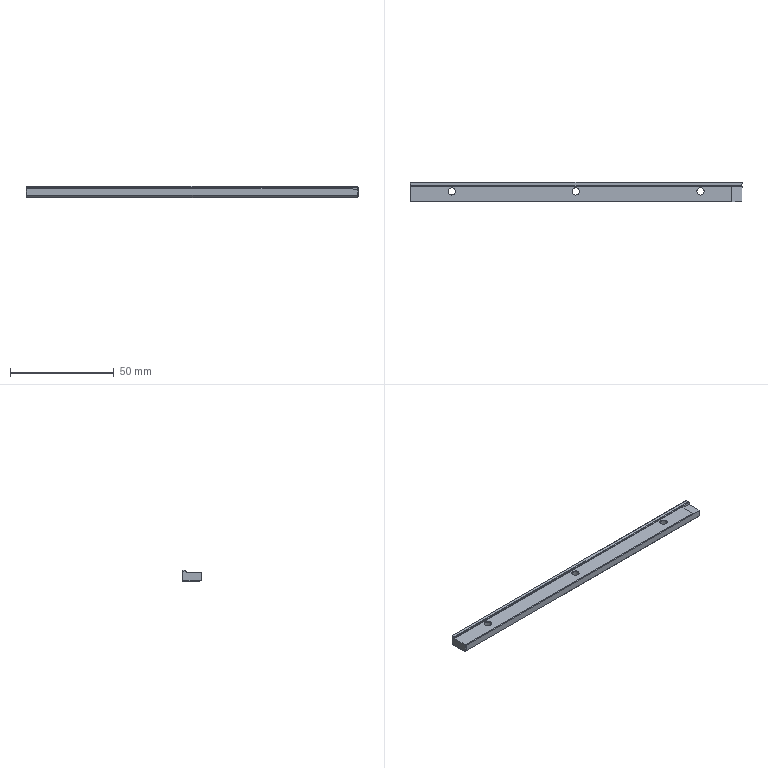Part | NX | 1 solid | 37 faces | box 159.75 x 9.6 x 5.3 mm | volume 6676 mm3 | plane 25 | cylinder 12 | commonest cylinder face diameters 3.5 x6 6 x6
STEP:
#1=CARTESIAN_POINT('',(13.59,-23.929,2.403));
#2=VERTEX_POINT('',#1);
#3=CARTESIAN_POINT('',(-145.56,-23.929,2.403));
#4=VERTEX_POINT('',#3);
#5=CARTESIAN_POINT('',(13.89,-23.929,2.403));
#6=DIRECTION('',(-1.,0.,0.));
#7=VECTOR('',#6,1000.);
#8=LINE('',#5,#7);
#9=EDGE_CURVE('',#2,#4,#8,.T.);
#10=ORIENTED_EDGE('',*,*,#9,.F.);
#11=CARTESIAN_POINT('',(13.59,-32.229,2.403));
#12=VERTEX_POINT('',#11);
#13=CARTESIAN_POINT('',(13.59,-27.929,2.403));
#14=DIRECTION('',(0.,1.,0.));
#15=VECTOR('',#14,1000.);
#16=LINE('',#13,#15);
#17=EDGE_CURVE('',#12,#2,#16,.T.);
#18=ORIENTED_EDGE('',*,*,#17,.F.);
#19=CARTESIAN_POINT('',(-145.56,-32.229,2.403));
#20=VERTEX_POINT('',#19);
#21=CARTESIAN_POINT('',(13.89,-32.229,2.403));
#22=DIRECTION('',(-1.,0.,0.));
#23=VECTOR('',#22,1000.);
#24=LINE('',#21,#23);
#25=EDGE_CURVE('',#12,#20,#24,.T.);
#26=ORIENTED_EDGE('',*,*,#25,.T.);
#27=CARTESIAN_POINT('',(-145.56,-28.079,2.403));
#28=DIRECTION('',(0.,-1.,0.));
#29=VECTOR('',#28,1000.);
#30=LINE('',#27,#29);
#31=EDGE_CURVE('',#4,#20,#30,.T.);
#32=ORIENTED_EDGE('',*,*,#31,.F.);
#33=EDGE_LOOP('',(#10,#18,#26,#32));
#34=FACE_BOUND('',#33,.T.);
#35=CARTESIAN_POINT('',(-66.11,-25.129,2.403));
#36=VERTEX_POINT('',#35);
#37=CARTESIAN_POINT('',(-66.11,-31.129,2.403));
#38=VERTEX_POINT('',#37);
#39=CARTESIAN_POINT('',(-66.11,-28.129,2.403));
#40=DIRECTION('',(0.,0.,-1.));
#41=DIRECTION('',(0.,-1.,0.));
#42=AXIS2_PLACEMENT_3D('',#39,#40,#41);
#43=CIRCLE('',#42,3.);
#44=EDGE_CURVE('',#36,#38,#43,.T.);
#45=ORIENTED_EDGE('',*,*,#44,.F.);
#46=CARTESIAN_POINT('',(-66.11,-28.129,2.403));
#47=DIRECTION('',(0.,0.,-1.));
#48=DIRECTION('',(0.,-1.,0.));
#49=AXIS2_PLACEMENT_3D('',#46,#47,#48);
#50=CIRCLE('',#49,3.);
#51=EDGE_CURVE('',#38,#36,#50,.T.);
#52=ORIENTED_EDGE('',*,*,#51,.F.);
#53=EDGE_LOOP('',(#45,#52));
#54=FACE_BOUND('',#53,.T.);
#55=CARTESIAN_POINT('',(-6.11,-25.129,2.403));
#56=VERTEX_POINT('',#55);
#57=CARTESIAN_POINT('',(-6.11,-31.129,2.403));
#58=VERTEX_POINT('',#57);
#59=CARTESIAN_POINT('',(-6.11,-28.129,2.403));
#60=DIRECTION('',(0.,0.,-1.));
#61=DIRECTION('',(0.,-1.,0.));
#62=AXIS2_PLACEMENT_3D('',#59,#60,#61);
#63=CIRCLE('',#62,3.);
#64=EDGE_CURVE('',#56,#58,#63,.T.);
#65=ORIENTED_EDGE('',*,*,#64,.F.);
#66=CARTESIAN_POINT('',(-6.11,-28.129,2.403));
#67=DIRECTION('',(0.,0.,-1.));
#68=DIRECTION('',(0.,-1.,0.));
#69=AXIS2_PLACEMENT_3D('',#66,#67,#68);
#70=CIRCLE('',#69,3.);
#71=EDGE_CURVE('',#58,#56,#70,.T.);
#72=ORIENTED_EDGE('',*,*,#71,.F.);
#73=EDGE_LOOP('',(#65,#72));
#74=FACE_BOUND('',#73,.T.);
#75=CARTESIAN_POINT('',(-125.709,-25.129,2.403));
#76=VERTEX_POINT('',#75);
#77=CARTESIAN_POINT('',(-125.709,-31.129,2.403));
#78=VERTEX_POINT('',#77);
#79=CARTESIAN_POINT('',(-125.709,-28.129,2.403));
#80=DIRECTION('',(0.,0.,-1.));
#81=DIRECTION('',(0.,-1.,0.));
#82=AXIS2_PLACEMENT_3D('',#79,#80,#81);
#83=CIRCLE('',#82,3.);
#84=EDGE_CURVE('',#76,#78,#83,.T.);
#85=ORIENTED_EDGE('',*,*,#84,.F.);
#86=CARTESIAN_POINT('',(-125.709,-28.129,2.403));
#87=DIRECTION('',(0.,0.,-1.));
#88=DIRECTION('',(0.,-1.,0.));
#89=AXIS2_PLACEMENT_3D('',#86,#87,#88);
#90=CIRCLE('',#89,3.);
#91=EDGE_CURVE('',#78,#76,#90,.T.);
#92=ORIENTED_EDGE('',*,*,#91,.F.);
#93=EDGE_LOOP('',(#85,#92));
#94=FACE_BOUND('',#93,.T.);
#95=CARTESIAN_POINT('',(13.89,-32.629,2.403));
#96=DIRECTION('',(0.,0.,-1.));
#97=DIRECTION('',(0.,-1.,0.));
#98=AXIS2_PLACEMENT_3D('',#95,#96,#97);
#99=PLANE('',#98);
#100=ADVANCED_FACE('',(#34,#54,#74,#94),#99,.T.);
#101=CARTESIAN_POINT('',(-145.56,-33.229,3.403));
#102=VERTEX_POINT('',#101);
#103=CARTESIAN_POINT('',(-145.56,-33.229,6.603));
#104=VERTEX_POINT('',#103);
#105=CARTESIAN_POINT('',(-145.56,-33.229,5.003));
#106=DIRECTION('',(0.,0.,1.));
#107=VECTOR('',#106,1000.);
#108=LINE('',#105,#107);
#109=EDGE_CURVE('',#102,#104,#108,.T.);
#110=ORIENTED_EDGE('',*,*,#109,.F.);
#111=CARTESIAN_POINT('',(13.59,-33.229,3.403));
#112=VERTEX_POINT('',#111);
#113=CARTESIAN_POINT('',(13.89,-33.229,3.403));
#114=DIRECTION('',(-1.,0.,0.));
#115=VECTOR('',#114,1000.);
#116=LINE('',#113,#115);
#117=EDGE_CURVE('',#112,#102,#116,.T.);
#118=ORIENTED_EDGE('',*,*,#117,.F.);
#119=CARTESIAN_POINT('',(13.59,-33.229,6.074));
#120=VERTEX_POINT('',#119);
#121=CARTESIAN_POINT('',(13.59,-33.229,4.712));
#122=DIRECTION('',(0.,0.,-1.));
#123=VECTOR('',#122,1000.);
#124=LINE('',#121,#123);
#125=EDGE_CURVE('',#120,#112,#124,.T.);
#126=ORIENTED_EDGE('',*,*,#125,.F.);
#127=CARTESIAN_POINT('',(10.591,-33.229,6.603));
#128=VERTEX_POINT('',#127);
#129=CARTESIAN_POINT('',(13.89,-33.229,6.021));
#130=DIRECTION('',(0.9848,0.,-0.1736));
#131=VECTOR('',#130,1000.);
#132=LINE('',#129,#131);
#133=EDGE_CURVE('',#128,#120,#132,.T.);
#134=ORIENTED_EDGE('',*,*,#133,.F.);
#135=CARTESIAN_POINT('',(13.89,-33.229,6.603));
#136=DIRECTION('',(1.,0.,0.));
#137=VECTOR('',#136,1000.);
#138=LINE('',#135,#137);
#139=EDGE_CURVE('',#104,#128,#138,.T.);
#140=ORIENTED_EDGE('',*,*,#139,.F.);
#141=EDGE_LOOP('',(#110,#118,#126,#134,#140));
#142=FACE_BOUND('',#141,.T.);
#143=CARTESIAN_POINT('',(13.89,-33.229,6.903));
#144=DIRECTION('',(0.,-1.,0.));
#145=DIRECTION('',(-1.,0.,0.));
#146=AXIS2_PLACEMENT_3D('',#143,#144,#145);
#147=PLANE('',#146);
#148=ADVANCED_FACE('',(#142),#147,.T.);
#149=CARTESIAN_POINT('',(8.89,-25.629,6.903));
#150=VERTEX_POINT('',#149);
#151=CARTESIAN_POINT('',(8.89,-32.929,6.903));
#152=VERTEX_POINT('',#151);
#153=CARTESIAN_POINT('',(8.89,-28.565,6.903));
#154=DIRECTION('',(0.,-1.,0.));
#155=VECTOR('',#154,1000.);
#156=LINE('',#153,#155);
#157=EDGE_CURVE('',#150,#152,#156,.T.);
#158=ORIENTED_EDGE('',*,*,#157,.F.);
#159=CARTESIAN_POINT('',(-145.86,-25.629,6.903));
#160=VERTEX_POINT('',#159);
#161=CARTESIAN_POINT('',(13.89,-25.629,6.903));
#162=DIRECTION('',(1.,0.,0.));
#163=VECTOR('',#162,1000.);
#164=LINE('',#161,#163);
#165=EDGE_CURVE('',#160,#150,#164,.T.);
#166=ORIENTED_EDGE('',*,*,#165,.F.);
#167=CARTESIAN_POINT('',(-145.86,-32.929,6.903));
#168=VERTEX_POINT('',#167);
#169=CARTESIAN_POINT('',(-145.86,-28.565,6.903));
#170=DIRECTION('',(0.,1.,0.));
#171=VECTOR('',#170,1000.);
#172=LINE('',#169,#171);
#173=EDGE_CURVE('',#168,#160,#172,.T.);
#174=ORIENTED_EDGE('',*,*,#173,.F.);
#175=CARTESIAN_POINT('',(13.89,-32.929,6.903));
#176=DIRECTION('',(1.,0.,0.));
#177=VECTOR('',#176,1000.);
#178=LINE('',#175,#177);
#179=EDGE_CURVE('',#168,#152,#178,.T.);
#180=ORIENTED_EDGE('',*,*,#179,.T.);
#181=EDGE_LOOP('',(#158,#166,#174,#180));
#182=FACE_BOUND('',#181,.T.);
#183=CARTESIAN_POINT('',(-125.709,-26.379,6.903));
#184=VERTEX_POINT('',#183);
#185=CARTESIAN_POINT('',(-125.709,-29.879,6.903));
#186=VERTEX_POINT('',#185);
#187=CARTESIAN_POINT('',(-125.709,-28.129,6.903));
#188=DIRECTION('',(0.,0.,-1.));
#189=DIRECTION('',(0.,-1.,0.));
#190=AXIS2_PLACEMENT_3D('',#187,#188,#189);
#191=CIRCLE('',#190,1.75);
#192=EDGE_CURVE('',#184,#186,#191,.T.);
#193=ORIENTED_EDGE('',*,*,#192,.T.);
#194=CARTESIAN_POINT('',(-125.709,-28.129,6.903));
#195=DIRECTION('',(0.,0.,-1.));
#196=DIRECTION('',(0.,-1.,0.));
#197=AXIS2_PLACEMENT_3D('',#194,#195,#196);
#198=CIRCLE('',#197,1.75);
#199=EDGE_CURVE('',#186,#184,#198,.T.);
#200=ORIENTED_EDGE('',*,*,#199,.T.);
#201=EDGE_LOOP('',(#193,#200));
#202=FACE_BOUND('',#201,.T.);
#203=CARTESIAN_POINT('',(-6.11,-26.379,6.903));
#204=VERTEX_POINT('',#203);
#205=CARTESIAN_POINT('',(-6.11,-29.879,6.903));
#206=VERTEX_POINT('',#205);
#207=CARTESIAN_POINT('',(-6.11,-28.129,6.903));
#208=DIRECTION('',(0.,0.,-1.));
#209=DIRECTION('',(0.,-1.,0.));
#210=AXIS2_PLACEMENT_3D('',#207,#208,#209);
#211=CIRCLE('',#210,1.75);
#212=EDGE_CURVE('',#204,#206,#211,.T.);
#213=ORIENTED_EDGE('',*,*,#212,.T.);
#214=CARTESIAN_POINT('',(-6.11,-28.129,6.903));
#215=DIRECTION('',(0.,0.,-1.));
#216=DIRECTION('',(0.,-1.,0.));
#217=AXIS2_PLACEMENT_3D('',#214,#215,#216);
#218=CIRCLE('',#217,1.75);
#219=EDGE_CURVE('',#206,#204,#218,.T.);
#220=ORIENTED_EDGE('',*,*,#219,.T.);
#221=EDGE_LOOP('',(#213,#220));
#222=FACE_BOUND('',#221,.T.);
#223=CARTESIAN_POINT('',(-66.11,-26.379,6.903));
#224=VERTEX_POINT('',#223);
#225=CARTESIAN_POINT('',(-66.11,-29.879,6.903));
#226=VERTEX_POINT('',#225);
#227=CARTESIAN_POINT('',(-66.11,-28.129,6.903));
#228=DIRECTION('',(0.,0.,-1.));
#229=DIRECTION('',(0.,-1.,0.));
#230=AXIS2_PLACEMENT_3D('',#227,#228,#229);
#231=CIRCLE('',#230,1.75);
#232=EDGE_CURVE('',#224,#226,#231,.T.);
#233=ORIENTED_EDGE('',*,*,#232,.T.);
#234=CARTESIAN_POINT('',(-66.11,-28.129,6.903));
#235=DIRECTION('',(0.,0.,-1.));
#236=DIRECTION('',(0.,-1.,0.));
#237=AXIS2_PLACEMENT_3D('',#234,#235,#236);
#238=CIRCLE('',#237,1.75);
#239=EDGE_CURVE('',#226,#224,#238,.T.);
#240=ORIENTED_EDGE('',*,*,#239,.T.);
#241=EDGE_LOOP('',(#233,#240));
#242=FACE_BOUND('',#241,.T.);
#243=CARTESIAN_POINT('',(13.89,-25.629,6.903));
#244=DIRECTION('',(0.,0.,1.));
#245=DIRECTION('',(1.,0.,0.));
#246=AXIS2_PLACEMENT_3D('',#243,#244,#245);
#247=PLANE('',#246);
#248=ADVANCED_FACE('',(#182,#202,#222,#242),#247,.T.);
#249=CARTESIAN_POINT('',(-145.56,-23.629,7.403));
#250=VERTEX_POINT('',#249);
#251=CARTESIAN_POINT('',(-145.56,-23.629,2.703));
#252=VERTEX_POINT('',#251);
#253=CARTESIAN_POINT('',(-145.56,-23.629,5.053));
#254=DIRECTION('',(0.,0.,-1.));
#255=VECTOR('',#254,1000.);
#256=LINE('',#253,#255);
#257=EDGE_CURVE('',#250,#252,#256,.T.);
#258=ORIENTED_EDGE('',*,*,#257,.F.);
#259=CARTESIAN_POINT('',(13.59,-23.629,7.403));
#260=VERTEX_POINT('',#259);
#261=CARTESIAN_POINT('',(13.89,-23.629,7.403));
#262=DIRECTION('',(-1.,0.,0.));
#263=VECTOR('',#262,1000.);
#264=LINE('',#261,#263);
#265=EDGE_CURVE('',#260,#250,#264,.T.);
#266=ORIENTED_EDGE('',*,*,#265,.F.);
#267=CARTESIAN_POINT('',(13.59,-23.629,2.703));
#268=VERTEX_POINT('',#267);
#269=CARTESIAN_POINT('',(13.59,-23.629,5.053));
#270=DIRECTION('',(0.,0.,1.));
#271=VECTOR('',#270,1000.);
#272=LINE('',#269,#271);
#273=EDGE_CURVE('',#268,#260,#272,.T.);
#274=ORIENTED_EDGE('',*,*,#273,.F.);
#275=CARTESIAN_POINT('',(13.89,-23.629,2.703));
#276=DIRECTION('',(-1.,0.,0.));
#277=VECTOR('',#276,1000.);
#278=LINE('',#275,#277);
#279=EDGE_CURVE('',#268,#252,#278,.T.);
#280=ORIENTED_EDGE('',*,*,#279,.T.);
#281=EDGE_LOOP('',(#258,#266,#274,#280));
#282=FACE_BOUND('',#281,.T.);
#283=CARTESIAN_POINT('',(13.89,-23.629,4.403));
#284=DIRECTION('',(0.,1.,0.));
#285=DIRECTION('',(1.,0.,0.));
#286=AXIS2_PLACEMENT_3D('',#283,#284,#285);
#287=PLANE('',#286);
#288=ADVANCED_FACE('',(#282),#287,.T.);
#289=ORIENTED_EDGE('',*,*,#64,.T.);
#290=CARTESIAN_POINT('',(-6.11,-31.129,6.403));
#291=VERTEX_POINT('',#290);
#292=CARTESIAN_POINT('',(-6.11,-31.129,3.403));
#293=DIRECTION('',(0.,0.,-1.));
#294=VECTOR('',#293,1000.);
#295=LINE('',#292,#294);
#296=EDGE_CURVE('',#58,#291,#295,.F.);
#297=ORIENTED_EDGE('',*,*,#296,.T.);
#298=CARTESIAN_POINT('',(-6.11,-25.129,6.403));
#299=VERTEX_POINT('',#298);
#300=CARTESIAN_POINT('',(-6.11,-28.129,6.403));
#301=DIRECTION('',(0.,0.,-1.));
#302=DIRECTION('',(0.,-1.,0.));
#303=AXIS2_PLACEMENT_3D('',#300,#301,#302);
#304=CIRCLE('',#303,3.);
#305=EDGE_CURVE('',#299,#291,#304,.T.);
#306=ORIENTED_EDGE('',*,*,#305,.F.);
#307=CARTESIAN_POINT('',(-6.11,-25.129,3.403));
#308=DIRECTION('',(0.,0.,-1.));
#309=VECTOR('',#308,1000.);
#310=LINE('',#307,#309);
#311=EDGE_CURVE('',#56,#299,#310,.F.);
#312=ORIENTED_EDGE('',*,*,#311,.F.);
#313=EDGE_LOOP('',(#289,#297,#306,#312));
#314=FACE_BOUND('',#313,.T.);
#315=CARTESIAN_POINT('',(-6.11,-28.129,3.403));
#316=DIRECTION('',(0.,0.,-1.));
#317=DIRECTION('',(0.,-1.,0.));
#318=AXIS2_PLACEMENT_3D('',#315,#316,#317);
#319=CYLINDRICAL_SURFACE('',#318,3.);
#320=ADVANCED_FACE('',(#314),#319,.F.);
#321=ORIENTED_EDGE('',*,*,#305,.T.);
#322=CARTESIAN_POINT('',(-6.11,-28.129,6.403));
#323=DIRECTION('',(0.,0.,-1.));
#324=DIRECTION('',(0.,-1.,0.));
#325=AXIS2_PLACEMENT_3D('',#322,#323,#324);
#326=CIRCLE('',#325,3.);
#327=EDGE_CURVE('',#291,#299,#326,.T.);
#328=ORIENTED_EDGE('',*,*,#327,.T.);
#329=EDGE_LOOP('',(#321,#328));
#330=FACE_BOUND('',#329,.T.);
#331=CARTESIAN_POINT('',(-6.11,-26.379,6.403));
#332=VERTEX_POINT('',#331);
#333=CARTESIAN_POINT('',(-6.11,-29.879,6.403));
#334=VERTEX_POINT('',#333);
#335=CARTESIAN_POINT('',(-6.11,-28.129,6.403));
#336=DIRECTION('',(0.,0.,-1.));
#337=DIRECTION('',(0.,-1.,0.));
#338=AXIS2_PLACEMENT_3D('',#335,#336,#337);
#339=CIRCLE('',#338,1.75);
#340=EDGE_CURVE('',#332,#334,#339,.T.);
#341=ORIENTED_EDGE('',*,*,#340,.F.);
#342=CARTESIAN_POINT('',(-6.11,-28.129,6.403));
#343=DIRECTION('',(0.,0.,-1.));
#344=DIRECTION('',(0.,-1.,0.));
#345=AXIS2_PLACEMENT_3D('',#342,#343,#344);
#346=CIRCLE('',#345,1.75);
#347=EDGE_CURVE('',#334,#332,#346,.T.);
#348=ORIENTED_EDGE('',*,*,#347,.F.);
#349=EDGE_LOOP('',(#341,#348));
#350=FACE_BOUND('',#349,.T.);
#351=CARTESIAN_POINT('',(-6.11,-28.129,6.403));
#352=DIRECTION('',(0.,0.,-1.));
#353=DIRECTION('',(0.,-1.,0.));
#354=AXIS2_PLACEMENT_3D('',#351,#352,#353);
#355=PLANE('',#354);
#356=ADVANCED_FACE('',(#330,#350),#355,.T.);
#357=ORIENTED_EDGE('',*,*,#340,.T.);
#358=CARTESIAN_POINT('',(-6.11,-29.879,3.403));
#359=DIRECTION('',(0.,0.,-1.));
#360=VECTOR('',#359,1000.);
#361=LINE('',#358,#360);
#362=EDGE_CURVE('',#334,#206,#361,.F.);
#363=ORIENTED_EDGE('',*,*,#362,.T.);
#364=ORIENTED_EDGE('',*,*,#212,.F.);
#365=CARTESIAN_POINT('',(-6.11,-26.379,3.403));
#366=DIRECTION('',(0.,0.,-1.));
#367=VECTOR('',#366,1000.);
#368=LINE('',#365,#367);
#369=EDGE_CURVE('',#332,#204,#368,.F.);
#370=ORIENTED_EDGE('',*,*,#369,.F.);
#371=EDGE_LOOP('',(#357,#363,#364,#370));
#372=FACE_BOUND('',#371,.T.);
#373=CARTESIAN_POINT('',(-6.11,-28.129,3.403));
#374=DIRECTION('',(0.,0.,-1.));
#375=DIRECTION('',(0.,-1.,0.));
#376=AXIS2_PLACEMENT_3D('',#373,#374,#375);
#377=CYLINDRICAL_SURFACE('',#376,1.75);
#378=ADVANCED_FACE('',(#372),#377,.F.);
#379=CARTESIAN_POINT('',(-66.11,-26.379,6.403));
#380=VERTEX_POINT('',#379);
#381=CARTESIAN_POINT('',(-66.11,-29.879,6.403));
#382=VERTEX_POINT('',#381);
#383=CARTESIAN_POINT('',(-66.11,-28.129,6.403));
#384=DIRECTION('',(0.,0.,-1.));
#385=DIRECTION('',(0.,-1.,0.));
#386=AXIS2_PLACEMENT_3D('',#383,#384,#385);
#387=CIRCLE('',#386,1.75);
#388=EDGE_CURVE('',#380,#382,#387,.T.);
#389=ORIENTED_EDGE('',*,*,#388,.T.);
#390=CARTESIAN_POINT('',(-66.11,-29.879,3.403));
#391=DIRECTION('',(0.,0.,-1.));
#392=VECTOR('',#391,1000.);
#393=LINE('',#390,#392);
#394=EDGE_CURVE('',#382,#226,#393,.F.);
#395=ORIENTED_EDGE('',*,*,#394,.T.);
#396=ORIENTED_EDGE('',*,*,#232,.F.);
#397=CARTESIAN_POINT('',(-66.11,-26.379,3.403));
#398=DIRECTION('',(0.,0.,-1.));
#399=VECTOR('',#398,1000.);
#400=LINE('',#397,#399);
#401=EDGE_CURVE('',#380,#224,#400,.F.);
#402=ORIENTED_EDGE('',*,*,#401,.F.);
#403=EDGE_LOOP('',(#389,#395,#396,#402));
#404=FACE_BOUND('',#403,.T.);
#405=CARTESIAN_POINT('',(-66.11,-28.129,3.403));
#406=DIRECTION('',(0.,0.,-1.));
#407=DIRECTION('',(0.,-1.,0.));
#408=AXIS2_PLACEMENT_3D('',#405,#406,#407);
#409=CYLINDRICAL_SURFACE('',#408,1.75);
#410=ADVANCED_FACE('',(#404),#409,.F.);
#411=CARTESIAN_POINT('',(-66.11,-25.129,6.403));
#412=VERTEX_POINT('',#411);
#413=CARTESIAN_POINT('',(-66.11,-31.129,6.403));
#414=VERTEX_POINT('',#413);
#415=CARTESIAN_POINT('',(-66.11,-28.129,6.403));
#416=DIRECTION('',(0.,0.,-1.));
#417=DIRECTION('',(0.,-1.,0.));
#418=AXIS2_PLACEMENT_3D('',#415,#416,#417);
#419=CIRCLE('',#418,3.);
#420=EDGE_CURVE('',#412,#414,#419,.T.);
#421=ORIENTED_EDGE('',*,*,#420,.T.);
#422=CARTESIAN_POINT('',(-66.11,-28.129,6.403));
#423=DIRECTION('',(0.,0.,-1.));
#424=DIRECTION('',(0.,-1.,0.));
#425=AXIS2_PLACEMENT_3D('',#422,#423,#424);
#426=CIRCLE('',#425,3.);
#427=EDGE_CURVE('',#414,#412,#426,.T.);
#428=ORIENTED_EDGE('',*,*,#427,.T.);
#429=EDGE_LOOP('',(#421,#428));
#430=FACE_BOUND('',#429,.T.);
#431=ORIENTED_EDGE('',*,*,#388,.F.);
#432=CARTESIAN_POINT('',(-66.11,-28.129,6.403));
#433=DIRECTION('',(0.,0.,-1.));
#434=DIRECTION('',(0.,-1.,0.));
#435=AXIS2_PLACEMENT_3D('',#432,#433,#434);
#436=CIRCLE('',#435,1.75);
#437=EDGE_CURVE('',#382,#380,#436,.T.);
#438=ORIENTED_EDGE('',*,*,#437,.F.);
#439=EDGE_LOOP('',(#431,#438));
#440=FACE_BOUND('',#439,.T.);
#441=CARTESIAN_POINT('',(-66.11,-28.129,6.403));
#442=DIRECTION('',(0.,0.,-1.));
#443=DIRECTION('',(0.,-1.,0.));
#444=AXIS2_PLACEMENT_3D('',#441,#442,#443);
#445=PLANE('',#444);
#446=ADVANCED_FACE('',(#430,#440),#445,.T.);
#447=ORIENTED_EDGE('',*,*,#44,.T.);
#448=CARTESIAN_POINT('',(-66.11,-31.129,3.403));
#449=DIRECTION('',(0.,0.,-1.));
#450=VECTOR('',#449,1000.);
#451=LINE('',#448,#450);
#452=EDGE_CURVE('',#38,#414,#451,.F.);
#453=ORIENTED_EDGE('',*,*,#452,.T.);
#454=ORIENTED_EDGE('',*,*,#420,.F.);
#455=CARTESIAN_POINT('',(-66.11,-25.129,3.403));
#456=DIRECTION('',(0.,0.,-1.));
#457=VECTOR('',#456,1000.);
#458=LINE('',#455,#457);
#459=EDGE_CURVE('',#36,#412,#458,.F.);
#460=ORIENTED_EDGE('',*,*,#459,.F.);
#461=EDGE_LOOP('',(#447,#453,#454,#460));
#462=FACE_BOUND('',#461,.T.);
#463=CARTESIAN_POINT('',(-66.11,-28.129,3.403));
#464=DIRECTION('',(0.,0.,-1.));
#465=DIRECTION('',(0.,-1.,0.));
#466=AXIS2_PLACEMENT_3D('',#463,#464,#465);
#467=CYLINDRICAL_SURFACE('',#466,3.);
#468=ADVANCED_FACE('',(#462),#467,.F.);
#469=CARTESIAN_POINT('',(-125.709,-26.379,6.403));
#470=VERTEX_POINT('',#469);
#471=CARTESIAN_POINT('',(-125.709,-29.879,6.403));
#472=VERTEX_POINT('',#471);
#473=CARTESIAN_POINT('',(-125.709,-28.129,6.403));
#474=DIRECTION('',(0.,0.,-1.));
#475=DIRECTION('',(0.,-1.,0.));
#476=AXIS2_PLACEMENT_3D('',#473,#474,#475);
#477=CIRCLE('',#476,1.75);
#478=EDGE_CURVE('',#470,#472,#477,.T.);
#479=ORIENTED_EDGE('',*,*,#478,.T.);
#480=CARTESIAN_POINT('',(-125.709,-29.879,3.403));
#481=DIRECTION('',(0.,0.,-1.));
#482=VECTOR('',#481,1000.);
#483=LINE('',#480,#482);
#484=EDGE_CURVE('',#472,#186,#483,.F.);
#485=ORIENTED_EDGE('',*,*,#484,.T.);
#486=ORIENTED_EDGE('',*,*,#192,.F.);
#487=CARTESIAN_POINT('',(-125.709,-26.379,3.403));
#488=DIRECTION('',(0.,0.,-1.));
#489=VECTOR('',#488,1000.);
#490=LINE('',#487,#489);
#491=EDGE_CURVE('',#470,#184,#490,.F.);
#492=ORIENTED_EDGE('',*,*,#491,.F.);
#493=EDGE_LOOP('',(#479,#485,#486,#492));
#494=FACE_BOUND('',#493,.T.);
#495=CARTESIAN_POINT('',(-125.709,-28.129,3.403));
#496=DIRECTION('',(0.,0.,-1.));
#497=DIRECTION('',(0.,-1.,0.));
#498=AXIS2_PLACEMENT_3D('',#495,#496,#497);
#499=CYLINDRICAL_SURFACE('',#498,1.75);
#500=ADVANCED_FACE('',(#494),#499,.F.);
#501=CARTESIAN_POINT('',(-125.709,-25.129,6.403));
#502=VERTEX_POINT('',#501);
#503=CARTESIAN_POINT('',(-125.709,-31.129,6.403));
#504=VERTEX_POINT('',#503);
#505=CARTESIAN_POINT('',(-125.709,-28.129,6.403));
#506=DIRECTION('',(0.,0.,-1.));
#507=DIRECTION('',(0.,-1.,0.));
#508=AXIS2_PLACEMENT_3D('',#505,#506,#507);
#509=CIRCLE('',#508,3.);
#510=EDGE_CURVE('',#502,#504,#509,.T.);
#511=ORIENTED_EDGE('',*,*,#510,.T.);
#512=CARTESIAN_POINT('',(-125.709,-28.129,6.403));
#513=DIRECTION('',(0.,0.,-1.));
#514=DIRECTION('',(0.,-1.,0.));
#515=AXIS2_PLACEMENT_3D('',#512,#513,#514);
#516=CIRCLE('',#515,3.);
#517=EDGE_CURVE('',#504,#502,#516,.T.);
#518=ORIENTED_EDGE('',*,*,#517,.T.);
#519=EDGE_LOOP('',(#511,#518));
#520=FACE_BOUND('',#519,.T.);
#521=ORIENTED_EDGE('',*,*,#478,.F.);
#522=CARTESIAN_POINT('',(-125.709,-28.129,6.403));
#523=DIRECTION('',(0.,0.,-1.));
#524=DIRECTION('',(0.,-1.,0.));
#525=AXIS2_PLACEMENT_3D('',#522,#523,#524);
#526=CIRCLE('',#525,1.75);
#527=EDGE_CURVE('',#472,#470,#526,.T.);
#528=ORIENTED_EDGE('',*,*,#527,.F.);
#529=EDGE_LOOP('',(#521,#528));
#530=FACE_BOUND('',#529,.T.);
#531=CARTESIAN_POINT('',(-125.709,-28.129,6.403));
#532=DIRECTION('',(0.,0.,-1.));
#533=DIRECTION('',(0.,-1.,0.));
#534=AXIS2_PLACEMENT_3D('',#531,#532,#533);
#535=PLANE('',#534);
#536=ADVANCED_FACE('',(#520,#530),#535,.T.);
#537=ORIENTED_EDGE('',*,*,#84,.T.);
#538=CARTESIAN_POINT('',(-125.709,-31.129,3.403));
#539=DIRECTION('',(0.,0.,-1.));
#540=VECTOR('',#539,1000.);
#541=LINE('',#538,#540);
#542=EDGE_CURVE('',#78,#504,#541,.F.);
#543=ORIENTED_EDGE('',*,*,#542,.T.);
#544=ORIENTED_EDGE('',*,*,#510,.F.);
#545=CARTESIAN_POINT('',(-125.709,-25.129,3.403));
#546=DIRECTION('',(0.,0.,-1.));
#547=VECTOR('',#546,1000.);
#548=LINE('',#545,#547);
#549=EDGE_CURVE('',#76,#502,#548,.F.);
#550=ORIENTED_EDGE('',*,*,#549,.F.);
#551=EDGE_LOOP('',(#537,#543,#544,#550));
#552=FACE_BOUND('',#551,.T.);
#553=CARTESIAN_POINT('',(-125.709,-28.129,3.403));
#554=DIRECTION('',(0.,0.,-1.));
#555=DIRECTION('',(0.,-1.,0.));
#556=AXIS2_PLACEMENT_3D('',#553,#554,#555);
#557=CYLINDRICAL_SURFACE('',#556,3.);
#558=ADVANCED_FACE('',(#552),#557,.F.);
#559=CARTESIAN_POINT('',(-145.56,-25.329,7.703));
#560=VERTEX_POINT('',#559);
#561=CARTESIAN_POINT('',(-145.56,-23.929,7.703));
#562=VERTEX_POINT('',#561);
#563=CARTESIAN_POINT('',(-145.56,-24.629,7.703));
#564=DIRECTION('',(0.,1.,0.));
#565=VECTOR('',#564,1000.);
#566=LINE('',#563,#565);
#567=EDGE_CURVE('',#560,#562,#566,.T.);
#568=ORIENTED_EDGE('',*,*,#567,.F.);
#569=CARTESIAN_POINT('',(13.59,-25.329,7.703));
#570=VERTEX_POINT('',#569);
#571=CARTESIAN_POINT('',(13.89,-25.329,7.703));
#572=DIRECTION('',(-1.,0.,0.));
#573=VECTOR('',#572,1000.);
#574=LINE('',#571,#573);
#575=EDGE_CURVE('',#570,#560,#574,.T.);
#576=ORIENTED_EDGE('',*,*,#575,.F.);
#577=CARTESIAN_POINT('',(13.59,-23.929,7.703));
#578=VERTEX_POINT('',#577);
#579=CARTESIAN_POINT('',(13.59,-24.629,7.703));
#580=DIRECTION('',(0.,-1.,0.));
#581=VECTOR('',#580,1000.);
#582=LINE('',#579,#581);
#583=EDGE_CURVE('',#578,#570,#582,.T.);
#584=ORIENTED_EDGE('',*,*,#583,.F.);
#585=CARTESIAN_POINT('',(13.89,-23.929,7.703));
#586=DIRECTION('',(-1.,0.,0.));
#587=VECTOR('',#586,1000.);
#588=LINE('',#585,#587);
#589=EDGE_CURVE('',#578,#562,#588,.T.);
#590=ORIENTED_EDGE('',*,*,#589,.T.);
#591=EDGE_LOOP('',(#568,#576,#584,#590));
#592=FACE_BOUND('',#591,.T.);
#593=CARTESIAN_POINT('',(-2.359,-25.191,7.703));
#594=DIRECTION('',(0.,0.,1.));
#595=DIRECTION('',(1.,0.,0.));
#596=AXIS2_PLACEMENT_3D('',#593,#594,#595);
#597=PLANE('',#596);
#598=ADVANCED_FACE('',(#592),#597,.T.);
#599=ORIENTED_EDGE('',*,*,#165,.T.);
#600=CARTESIAN_POINT('',(13.89,-25.629,6.021));
#601=VERTEX_POINT('',#600);
#602=CARTESIAN_POINT('',(13.89,-25.629,6.021));
#603=DIRECTION('',(0.9848,0.,-0.1736));
#604=VECTOR('',#603,1000.);
#605=LINE('',#602,#604);
#606=EDGE_CURVE('',#150,#601,#605,.T.);
#607=ORIENTED_EDGE('',*,*,#606,.T.);
#608=CARTESIAN_POINT('',(13.89,-25.629,7.403));
#609=VERTEX_POINT('',#608);
#610=CARTESIAN_POINT('',(13.89,-25.629,11.359));
#611=DIRECTION('',(0.,0.,1.));
#612=VECTOR('',#611,1000.);
#613=LINE('',#610,#612);
#614=EDGE_CURVE('',#601,#609,#613,.T.);
#615=ORIENTED_EDGE('',*,*,#614,.T.);
#616=CARTESIAN_POINT('',(-145.86,-25.629,7.403));
#617=VERTEX_POINT('',#616);
#618=CARTESIAN_POINT('',(13.89,-25.629,7.403));
#619=DIRECTION('',(-1.,0.,0.));
#620=VECTOR('',#619,1000.);
#621=LINE('',#618,#620);
#622=EDGE_CURVE('',#609,#617,#621,.T.);
#623=ORIENTED_EDGE('',*,*,#622,.T.);
#624=CARTESIAN_POINT('',(-145.86,-25.629,11.359));
#625=DIRECTION('',(0.,0.,1.));
#626=VECTOR('',#625,1000.);
#627=LINE('',#624,#626);
#628=EDGE_CURVE('',#160,#617,#627,.T.);
#629=ORIENTED_EDGE('',*,*,#628,.F.);
#630=EDGE_LOOP('',(#599,#607,#615,#623,#629));
#631=FACE_BOUND('',#630,.T.);
#632=CARTESIAN_POINT('',(13.89,-25.629,6.903));
#633=DIRECTION('',(0.,-1.,0.));
#634=DIRECTION('',(0.,0.,-1.));
#635=AXIS2_PLACEMENT_3D('',#632,#633,#634);
#636=PLANE('',#635);
#637=ADVANCED_FACE('',(#631),#636,.T.);
#638=ORIENTED_EDGE('',*,*,#117,.T.);
#639=CARTESIAN_POINT('',(-145.86,-32.929,3.103));
#640=VERTEX_POINT('',#639);
#641=CARTESIAN_POINT('',(13.89,-192.679,162.853));
#642=DIRECTION('',(-0.5774,0.5774,-0.5774));
#643=VECTOR('',#642,1000.);
#644=LINE('',#641,#643);
#645=EDGE_CURVE('',#102,#640,#644,.T.);
#646=ORIENTED_EDGE('',*,*,#645,.T.);
#647=CARTESIAN_POINT('',(-145.86,-32.529,2.703));
#648=VERTEX_POINT('',#647);
#649=CARTESIAN_POINT('',(-145.86,-41.185,11.359));
#650=DIRECTION('',(0.,0.7071,-0.7071));
#651=VECTOR('',#650,1000.);
#652=LINE('',#649,#651);
#653=EDGE_CURVE('',#640,#648,#652,.T.);
#654=ORIENTED_EDGE('',*,*,#653,.T.);
#655=CARTESIAN_POINT('',(13.89,127.221,-157.047));
#656=DIRECTION('',(0.5774,0.5774,-0.5774));
#657=VECTOR('',#656,1000.);
#658=LINE('',#655,#657);
#659=EDGE_CURVE('',#648,#20,#658,.T.);
#660=ORIENTED_EDGE('',*,*,#659,.T.);
#661=ORIENTED_EDGE('',*,*,#25,.F.);
#662=CARTESIAN_POINT('',(13.89,-32.529,2.703));
#663=VERTEX_POINT('',#662);
#664=CARTESIAN_POINT('',(22.546,-41.185,11.359));
#665=DIRECTION('',(0.5774,-0.5774,0.5774));
#666=VECTOR('',#665,1000.);
#667=LINE('',#664,#666);
#668=EDGE_CURVE('',#12,#663,#667,.T.);
#669=ORIENTED_EDGE('',*,*,#668,.T.);
#670=CARTESIAN_POINT('',(13.89,-32.929,3.103));
#671=VERTEX_POINT('',#670);
#672=CARTESIAN_POINT('',(13.89,-41.185,11.359));
#673=DIRECTION('',(0.,0.7071,-0.7071));
#674=VECTOR('',#673,1000.);
#675=LINE('',#672,#674);
#676=EDGE_CURVE('',#671,#663,#675,.T.);
#677=ORIENTED_EDGE('',*,*,#676,.F.);
#678=CARTESIAN_POINT('',(13.89,-32.929,3.103));
#679=DIRECTION('',(-0.5774,-0.5774,0.5774));
#680=VECTOR('',#679,1000.);
#681=LINE('',#678,#680);
#682=EDGE_CURVE('',#671,#112,#681,.T.);
#683=ORIENTED_EDGE('',*,*,#682,.T.);
#684=EDGE_LOOP('',(#638,#646,#654,#660,#661,#669,#677,#683));
#685=FACE_BOUND('',#684,.T.);
#686=CARTESIAN_POINT('',(-65.61,-32.729,2.903));
#687=DIRECTION('',(0.,0.7071,0.7071));
#688=DIRECTION('',(1.,0.,0.));
#689=AXIS2_PLACEMENT_3D('',#686,#687,#688);
#690=PLANE('',#689);
#691=ADVANCED_FACE('',(#685),#690,.F.);
#692=ORIENTED_EDGE('',*,*,#9,.T.);
#693=CARTESIAN_POINT('',(-145.71,-23.779,2.553));
#694=VERTEX_POINT('',#693);
#695=CARTESIAN_POINT('',(13.89,-183.379,-157.047));
#696=DIRECTION('',(-0.5774,0.5774,0.5774));
#697=VECTOR('',#696,1000.);
#698=LINE('',#695,#697);
#699=EDGE_CURVE('',#4,#694,#698,.T.);
#700=ORIENTED_EDGE('',*,*,#699,.T.);
#701=CARTESIAN_POINT('',(13.89,135.821,162.153));
#702=DIRECTION('',(-0.5774,-0.5774,-0.5774));
#703=VECTOR('',#702,1000.);
#704=LINE('',#701,#703);
#705=EDGE_CURVE('',#252,#694,#704,.T.);
#706=ORIENTED_EDGE('',*,*,#705,.F.);
#707=ORIENTED_EDGE('',*,*,#279,.F.);
#708=CARTESIAN_POINT('',(13.74,-23.779,2.553));
#709=VERTEX_POINT('',#708);
#710=CARTESIAN_POINT('',(13.89,-23.929,2.403));
#711=DIRECTION('',(-0.5774,0.5774,0.5774));
#712=VECTOR('',#711,1000.);
#713=LINE('',#710,#712);
#714=EDGE_CURVE('',#709,#268,#713,.T.);
#715=ORIENTED_EDGE('',*,*,#714,.F.);
#716=CARTESIAN_POINT('',(22.546,-14.973,11.359));
#717=DIRECTION('',(-0.5774,-0.5774,-0.5774));
#718=VECTOR('',#717,1000.);
#719=LINE('',#716,#718);
#720=EDGE_CURVE('',#709,#2,#719,.T.);
#721=ORIENTED_EDGE('',*,*,#720,.T.);
#722=EDGE_LOOP('',(#692,#700,#706,#707,#715,#721));
#723=FACE_BOUND('',#722,.T.);
#724=CARTESIAN_POINT('',(-65.61,-23.779,2.553));
#725=DIRECTION('',(0.,-0.7071,0.7071));
#726=DIRECTION('',(-1.,0.,0.));
#727=AXIS2_PLACEMENT_3D('',#724,#725,#726);
#728=PLANE('',#727);
#729=ADVANCED_FACE('',(#723),#728,.F.);
#730=ORIENTED_EDGE('',*,*,#179,.F.);
#731=CARTESIAN_POINT('',(13.89,-192.679,-152.847));
#732=DIRECTION('',(0.5774,-0.5774,-0.5774));
#733=VECTOR('',#732,1000.);
#734=LINE('',#731,#733);
#735=EDGE_CURVE('',#168,#104,#734,.T.);
#736=ORIENTED_EDGE('',*,*,#735,.T.);
#737=ORIENTED_EDGE('',*,*,#139,.T.);
#738=CARTESIAN_POINT('',(13.89,-33.811,6.021));
#739=DIRECTION('',(0.9703,-0.1711,-0.1711));
#740=VECTOR('',#739,1000.);
#741=LINE('',#738,#740);
#742=EDGE_CURVE('',#152,#128,#741,.T.);
#743=ORIENTED_EDGE('',*,*,#742,.F.);
#744=EDGE_LOOP('',(#730,#736,#737,#743));
#745=FACE_BOUND('',#744,.T.);
#746=CARTESIAN_POINT('',(-68.11,-33.079,6.753));
#747=DIRECTION('',(0.,0.7071,-0.7071));
#748=DIRECTION('',(-1.,0.,0.));
#749=AXIS2_PLACEMENT_3D('',#746,#747,#748);
#750=PLANE('',#749);
#751=ADVANCED_FACE('',(#745),#750,.F.);
#752=CARTESIAN_POINT('',(13.89,134.121,167.153));
#753=DIRECTION('',(0.5774,0.5774,0.5774));
#754=VECTOR('',#753,1000.);
#755=LINE('',#752,#754);
#756=EDGE_CURVE('',#617,#560,#755,.T.);
#757=ORIENTED_EDGE('',*,*,#756,.F.);
#758=ORIENTED_EDGE('',*,*,#622,.F.);
#759=CARTESIAN_POINT('',(13.89,-25.629,7.403));
#760=DIRECTION('',(-0.5774,0.5774,0.5774));
#761=VECTOR('',#760,1000.);
#762=LINE('',#759,#761);
#763=EDGE_CURVE('',#609,#570,#762,.T.);
#764=ORIENTED_EDGE('',*,*,#763,.T.);
#765=ORIENTED_EDGE('',*,*,#575,.T.);
#766=EDGE_LOOP('',(#757,#758,#764,#765));
#767=FACE_BOUND('',#766,.T.);
#768=CARTESIAN_POINT('',(-65.61,-25.479,7.553));
#769=DIRECTION('',(0.,0.7071,-0.7071));
#770=DIRECTION('',(-1.,0.,0.));
#771=AXIS2_PLACEMENT_3D('',#768,#769,#770);
#772=PLANE('',#771);
#773=ADVANCED_FACE('',(#767),#772,.F.);
#774=ORIENTED_EDGE('',*,*,#265,.T.);
#775=CARTESIAN_POINT('',(-145.71,-23.779,7.553));
#776=VERTEX_POINT('',#775);
#777=CARTESIAN_POINT('',(13.89,135.821,-152.047));
#778=DIRECTION('',(-0.5774,-0.5774,0.5774));
#779=VECTOR('',#778,1000.);
#780=LINE('',#777,#779);
#781=EDGE_CURVE('',#250,#776,#780,.T.);
#782=ORIENTED_EDGE('',*,*,#781,.T.);
#783=CARTESIAN_POINT('',(13.89,-183.379,167.153));
#784=DIRECTION('',(0.5774,-0.5774,0.5774));
#785=VECTOR('',#784,1000.);
#786=LINE('',#783,#785);
#787=EDGE_CURVE('',#776,#562,#786,.T.);
#788=ORIENTED_EDGE('',*,*,#787,.T.);
#789=ORIENTED_EDGE('',*,*,#589,.F.);
#790=CARTESIAN_POINT('',(13.74,-23.779,7.553));
#791=VERTEX_POINT('',#790);
#792=CARTESIAN_POINT('',(13.89,-23.629,7.403));
#793=DIRECTION('',(-0.5774,-0.5774,0.5774));
#794=VECTOR('',#793,1000.);
#795=LINE('',#792,#794);
#796=EDGE_CURVE('',#791,#578,#795,.T.);
#797=ORIENTED_EDGE('',*,*,#796,.F.);
#798=CARTESIAN_POINT('',(13.89,-23.929,7.703));
#799=DIRECTION('',(0.5774,-0.5774,0.5774));
#800=VECTOR('',#799,1000.);
#801=LINE('',#798,#800);
#802=EDGE_CURVE('',#260,#791,#801,.T.);
#803=ORIENTED_EDGE('',*,*,#802,.F.);
#804=EDGE_LOOP('',(#774,#782,#788,#789,#797,#803));
#805=FACE_BOUND('',#804,.T.);
#806=CARTESIAN_POINT('',(-65.61,-23.779,7.553));
#807=DIRECTION('',(0.,0.7071,0.7071));
#808=DIRECTION('',(1.,0.,0.));
#809=AXIS2_PLACEMENT_3D('',#806,#807,#808);
#810=PLANE('',#809);
#811=ADVANCED_FACE('',(#805),#810,.T.);
#812=ORIENTED_EDGE('',*,*,#583,.T.);
#813=ORIENTED_EDGE('',*,*,#763,.F.);
#814=CARTESIAN_POINT('',(13.89,-23.929,7.403));
#815=VERTEX_POINT('',#814);
#816=CARTESIAN_POINT('',(13.89,-24.629,7.403));
#817=DIRECTION('',(0.,-1.,0.));
#818=VECTOR('',#817,1000.);
#819=LINE('',#816,#818);
#820=EDGE_CURVE('',#815,#609,#819,.T.);
#821=ORIENTED_EDGE('',*,*,#820,.F.);
#822=CARTESIAN_POINT('',(13.89,-23.929,7.403));
#823=DIRECTION('',(-0.5774,0.5774,0.5774));
#824=VECTOR('',#823,1000.);
#825=LINE('',#822,#824);
#826=EDGE_CURVE('',#815,#791,#825,.T.);
#827=ORIENTED_EDGE('',*,*,#826,.T.);
#828=ORIENTED_EDGE('',*,*,#796,.T.);
#829=EDGE_LOOP('',(#812,#813,#821,#827,#828));
#830=FACE_BOUND('',#829,.T.);
#831=CARTESIAN_POINT('',(13.74,-24.629,7.553));
#832=DIRECTION('',(-0.7071,0.,-0.7071));
#833=DIRECTION('',(-0.7071,0.,0.7071));
#834=AXIS2_PLACEMENT_3D('',#831,#832,#833);
#835=PLANE('',#834);
#836=ADVANCED_FACE('',(#830),#835,.F.);
#837=ORIENTED_EDGE('',*,*,#257,.T.);
#838=ORIENTED_EDGE('',*,*,#705,.T.);
#839=CARTESIAN_POINT('',(-145.86,-23.929,2.703));
#840=VERTEX_POINT('',#839);
#841=CARTESIAN_POINT('',(13.89,135.821,-157.047));
#842=DIRECTION('',(0.5774,0.5774,-0.5774));
#843=VECTOR('',#842,1000.);
#844=LINE('',#841,#843);
#845=EDGE_CURVE('',#840,#694,#844,.T.);
#846=ORIENTED_EDGE('',*,*,#845,.F.);
#847=CARTESIAN_POINT('',(-145.86,-23.929,7.403));
#848=VERTEX_POINT('',#847);
#849=CARTESIAN_POINT('',(-145.86,-23.929,5.053));
#850=DIRECTION('',(0.,0.,-1.));
#851=VECTOR('',#850,1000.);
#852=LINE('',#849,#851);
#853=EDGE_CURVE('',#848,#840,#852,.T.);
#854=ORIENTED_EDGE('',*,*,#853,.F.);
#855=CARTESIAN_POINT('',(13.89,135.821,167.153));
#856=DIRECTION('',(-0.5774,-0.5774,-0.5774));
#857=VECTOR('',#856,1000.);
#858=LINE('',#855,#857);
#859=EDGE_CURVE('',#776,#848,#858,.T.);
#860=ORIENTED_EDGE('',*,*,#859,.F.);
#861=ORIENTED_EDGE('',*,*,#781,.F.);
#862=EDGE_LOOP('',(#837,#838,#846,#854,#860,#861));
#863=FACE_BOUND('',#862,.T.);
#864=CARTESIAN_POINT('',(-145.71,-23.779,5.053));
#865=DIRECTION('',(0.7071,-0.7071,0.));
#866=DIRECTION('',(0.,0.,-1.));
#867=AXIS2_PLACEMENT_3D('',#864,#865,#866);
#868=PLANE('',#867);
#869=ADVANCED_FACE('',(#863),#868,.F.);
#870=ORIENTED_EDGE('',*,*,#567,.T.);
#871=ORIENTED_EDGE('',*,*,#787,.F.);
#872=ORIENTED_EDGE('',*,*,#859,.T.);
#873=CARTESIAN_POINT('',(-145.86,-24.629,7.403));
#874=DIRECTION('',(0.,1.,0.));
#875=VECTOR('',#874,1000.);
#876=LINE('',#873,#875);
#877=EDGE_CURVE('',#617,#848,#876,.T.);
#878=ORIENTED_EDGE('',*,*,#877,.F.);
#879=ORIENTED_EDGE('',*,*,#756,.T.);
#880=EDGE_LOOP('',(#870,#871,#872,#878,#879));
#881=FACE_BOUND('',#880,.T.);
#882=CARTESIAN_POINT('',(-145.71,-24.629,7.553));
#883=DIRECTION('',(0.7071,0.,-0.7071));
#884=DIRECTION('',(0.,-1.,0.));
#885=AXIS2_PLACEMENT_3D('',#882,#883,#884);
#886=PLANE('',#885);
#887=ADVANCED_FACE('',(#881),#886,.F.);
#888=ORIENTED_EDGE('',*,*,#394,.F.);
#889=ORIENTED_EDGE('',*,*,#437,.T.);
#890=ORIENTED_EDGE('',*,*,#401,.T.);
#891=ORIENTED_EDGE('',*,*,#239,.F.);
#892=EDGE_LOOP('',(#888,#889,#890,#891));
#893=FACE_BOUND('',#892,.T.);
#894=CARTESIAN_POINT('',(-66.11,-28.129,3.403));
#895=DIRECTION('',(0.,0.,-1.));
#896=DIRECTION('',(0.,-1.,0.));
#897=AXIS2_PLACEMENT_3D('',#894,#895,#896);
#898=CYLINDRICAL_SURFACE('',#897,1.75);
#899=ADVANCED_FACE('',(#893),#898,.F.);
#900=ORIENTED_EDGE('',*,*,#484,.F.);
#901=ORIENTED_EDGE('',*,*,#527,.T.);
#902=ORIENTED_EDGE('',*,*,#491,.T.);
#903=ORIENTED_EDGE('',*,*,#199,.F.);
#904=EDGE_LOOP('',(#900,#901,#902,#903));
#905=FACE_BOUND('',#904,.T.);
#906=CARTESIAN_POINT('',(-125.709,-28.129,3.403));
#907=DIRECTION('',(0.,0.,-1.));
#908=DIRECTION('',(0.,-1.,0.));
#909=AXIS2_PLACEMENT_3D('',#906,#907,#908);
#910=CYLINDRICAL_SURFACE('',#909,1.75);
#911=ADVANCED_FACE('',(#905),#910,.F.);
#912=ORIENTED_EDGE('',*,*,#452,.F.);
#913=ORIENTED_EDGE('',*,*,#51,.T.);
#914=ORIENTED_EDGE('',*,*,#459,.T.);
#915=ORIENTED_EDGE('',*,*,#427,.F.);
#916=EDGE_LOOP('',(#912,#913,#914,#915));
#917=FACE_BOUND('',#916,.T.);
#918=CARTESIAN_POINT('',(-66.11,-28.129,3.403));
#919=DIRECTION('',(0.,0.,-1.));
#920=DIRECTION('',(0.,-1.,0.));
#921=AXIS2_PLACEMENT_3D('',#918,#919,#920);
#922=CYLINDRICAL_SURFACE('',#921,3.);
#923=ADVANCED_FACE('',(#917),#922,.F.);
#924=ORIENTED_EDGE('',*,*,#542,.F.);
#925=ORIENTED_EDGE('',*,*,#91,.T.);
#926=ORIENTED_EDGE('',*,*,#549,.T.);
#927=ORIENTED_EDGE('',*,*,#517,.F.);
#928=EDGE_LOOP('',(#924,#925,#926,#927));
#929=FACE_BOUND('',#928,.T.);
#930=CARTESIAN_POINT('',(-125.709,-28.129,3.403));
#931=DIRECTION('',(0.,0.,-1.));
#932=DIRECTION('',(0.,-1.,0.));
#933=AXIS2_PLACEMENT_3D('',#930,#931,#932);
#934=CYLINDRICAL_SURFACE('',#933,3.);
#935=ADVANCED_FACE('',(#929),#934,.F.);
#936=ORIENTED_EDGE('',*,*,#362,.F.);
#937=ORIENTED_EDGE('',*,*,#347,.T.);
#938=ORIENTED_EDGE('',*,*,#369,.T.);
#939=ORIENTED_EDGE('',*,*,#219,.F.);
#940=EDGE_LOOP('',(#936,#937,#938,#939));
#941=FACE_BOUND('',#940,.T.);
#942=CARTESIAN_POINT('',(-6.11,-28.129,3.403));
#943=DIRECTION('',(0.,0.,-1.));
#944=DIRECTION('',(0.,-1.,0.));
#945=AXIS2_PLACEMENT_3D('',#942,#943,#944);
#946=CYLINDRICAL_SURFACE('',#945,1.75);
#947=ADVANCED_FACE('',(#941),#946,.F.);
#948=ORIENTED_EDGE('',*,*,#296,.F.);
#949=ORIENTED_EDGE('',*,*,#71,.T.);
#950=ORIENTED_EDGE('',*,*,#311,.T.);
#951=ORIENTED_EDGE('',*,*,#327,.F.);
#952=EDGE_LOOP('',(#948,#949,#950,#951));
#953=FACE_BOUND('',#952,.T.);
#954=CARTESIAN_POINT('',(-6.11,-28.129,3.403));
#955=DIRECTION('',(0.,0.,-1.));
#956=DIRECTION('',(0.,-1.,0.));
#957=AXIS2_PLACEMENT_3D('',#954,#955,#956);
#958=CYLINDRICAL_SURFACE('',#957,3.);
#959=ADVANCED_FACE('',(#953),#958,.F.);
#960=CARTESIAN_POINT('',(-145.86,-32.929,5.003));
#961=DIRECTION('',(0.,0.,1.));
#962=VECTOR('',#961,1000.);
#963=LINE('',#960,#962);
#964=EDGE_CURVE('',#640,#168,#963,.T.);
#965=ORIENTED_EDGE('',*,*,#964,.T.);
#966=ORIENTED_EDGE('',*,*,#173,.T.);
#967=ORIENTED_EDGE('',*,*,#628,.T.);
#968=ORIENTED_EDGE('',*,*,#877,.T.);
#969=ORIENTED_EDGE('',*,*,#853,.T.);
#970=CARTESIAN_POINT('',(-145.86,-28.079,2.703));
#971=DIRECTION('',(0.,-1.,0.));
#972=VECTOR('',#971,1000.);
#973=LINE('',#970,#972);
#974=EDGE_CURVE('',#840,#648,#973,.T.);
#975=ORIENTED_EDGE('',*,*,#974,.T.);
#976=ORIENTED_EDGE('',*,*,#653,.F.);
#977=EDGE_LOOP('',(#965,#966,#967,#968,#969,#975,#976));
#978=FACE_BOUND('',#977,.T.);
#979=CARTESIAN_POINT('',(-145.86,-28.565,11.359));
#980=DIRECTION('',(1.,0.,0.));
#981=DIRECTION('',(0.,-1.,0.));
#982=AXIS2_PLACEMENT_3D('',#979,#980,#981);
#983=PLANE('',#982);
#984=ADVANCED_FACE('',(#978),#983,.F.);
#985=ORIENTED_EDGE('',*,*,#974,.F.);
#986=ORIENTED_EDGE('',*,*,#845,.T.);
#987=ORIENTED_EDGE('',*,*,#699,.F.);
#988=ORIENTED_EDGE('',*,*,#31,.T.);
#989=ORIENTED_EDGE('',*,*,#659,.F.);
#990=EDGE_LOOP('',(#985,#986,#987,#988,#989));
#991=FACE_BOUND('',#990,.T.);
#992=CARTESIAN_POINT('',(-145.71,-28.079,2.553));
#993=DIRECTION('',(-0.7071,0.,-0.7071));
#994=DIRECTION('',(-0.7071,0.,0.7071));
#995=AXIS2_PLACEMENT_3D('',#992,#993,#994);
#996=PLANE('',#995);
#997=ADVANCED_FACE('',(#991),#996,.T.);
#998=ORIENTED_EDGE('',*,*,#964,.F.);
#999=ORIENTED_EDGE('',*,*,#645,.F.);
#1000=ORIENTED_EDGE('',*,*,#109,.T.);
#1001=ORIENTED_EDGE('',*,*,#735,.F.);
#1002=EDGE_LOOP('',(#998,#999,#1000,#1001));
#1003=FACE_BOUND('',#1002,.T.);
#1004=CARTESIAN_POINT('',(-145.71,-33.079,5.003));
#1005=DIRECTION('',(-0.7071,-0.7071,0.));
#1006=DIRECTION('',(-0.7071,0.7071,0.));
#1007=AXIS2_PLACEMENT_3D('',#1004,#1005,#1006);
#1008=PLANE('',#1007);
#1009=ADVANCED_FACE('',(#1003),#1008,.T.);
#1010=CARTESIAN_POINT('',(13.89,-32.929,6.021));
#1011=VERTEX_POINT('',#1010);
#1012=CARTESIAN_POINT('',(13.89,-32.929,4.712));
#1013=DIRECTION('',(0.,0.,-1.));
#1014=VECTOR('',#1013,1000.);
#1015=LINE('',#1012,#1014);
#1016=EDGE_CURVE('',#1011,#671,#1015,.T.);
#1017=ORIENTED_EDGE('',*,*,#1016,.T.);
#1018=ORIENTED_EDGE('',*,*,#676,.T.);
#1019=CARTESIAN_POINT('',(13.89,-23.929,2.703));
#1020=VERTEX_POINT('',#1019);
#1021=CARTESIAN_POINT('',(13.89,-27.929,2.703));
#1022=DIRECTION('',(0.,1.,0.));
#1023=VECTOR('',#1022,1000.);
#1024=LINE('',#1021,#1023);
#1025=EDGE_CURVE('',#663,#1020,#1024,.T.);
#1026=ORIENTED_EDGE('',*,*,#1025,.T.);
#1027=CARTESIAN_POINT('',(13.89,-23.929,5.053));
#1028=DIRECTION('',(0.,0.,1.));
#1029=VECTOR('',#1028,1000.);
#1030=LINE('',#1027,#1029);
#1031=EDGE_CURVE('',#1020,#815,#1030,.T.);
#1032=ORIENTED_EDGE('',*,*,#1031,.T.);
#1033=ORIENTED_EDGE('',*,*,#820,.T.);
#1034=ORIENTED_EDGE('',*,*,#614,.F.);
#1035=CARTESIAN_POINT('',(13.89,-28.565,6.021));
#1036=DIRECTION('',(0.,-1.,0.));
#1037=VECTOR('',#1036,1000.);
#1038=LINE('',#1035,#1037);
#1039=EDGE_CURVE('',#601,#1011,#1038,.T.);
#1040=ORIENTED_EDGE('',*,*,#1039,.T.);
#1041=EDGE_LOOP('',(#1017,#1018,#1026,#1032,#1033,#1034,#1040));
#1042=FACE_BOUND('',#1041,.T.);
#1043=CARTESIAN_POINT('',(13.89,-28.565,11.359));
#1044=DIRECTION('',(1.,0.,0.));
#1045=DIRECTION('',(0.,-1.,0.));
#1046=AXIS2_PLACEMENT_3D('',#1043,#1044,#1045);
#1047=PLANE('',#1046);
#1048=ADVANCED_FACE('',(#1042),#1047,.T.);
#1049=ORIENTED_EDGE('',*,*,#1039,.F.);
#1050=ORIENTED_EDGE('',*,*,#606,.F.);
#1051=ORIENTED_EDGE('',*,*,#157,.T.);
#1052=ORIENTED_EDGE('',*,*,#742,.T.);
#1053=ORIENTED_EDGE('',*,*,#133,.T.);
#1054=CARTESIAN_POINT('',(13.89,-32.929,6.021));
#1055=DIRECTION('',(-0.7017,-0.7017,0.1237));
#1056=VECTOR('',#1055,1000.);
#1057=LINE('',#1054,#1056);
#1058=EDGE_CURVE('',#1011,#120,#1057,.T.);
#1059=ORIENTED_EDGE('',*,*,#1058,.F.);
#1060=EDGE_LOOP('',(#1049,#1050,#1051,#1052,#1053,#1059));
#1061=FACE_BOUND('',#1060,.T.);
#1062=CARTESIAN_POINT('',(11.39,-28.879,6.462));
#1063=DIRECTION('',(0.1736,0.,0.9848));
#1064=DIRECTION('',(0.,-1.,0.));
#1065=AXIS2_PLACEMENT_3D('',#1062,#1063,#1064);
#1066=PLANE('',#1065);
#1067=ADVANCED_FACE('',(#1061),#1066,.T.);
#1068=ORIENTED_EDGE('',*,*,#1025,.F.);
#1069=ORIENTED_EDGE('',*,*,#668,.F.);
#1070=ORIENTED_EDGE('',*,*,#17,.T.);
#1071=ORIENTED_EDGE('',*,*,#720,.F.);
#1072=CARTESIAN_POINT('',(22.546,-32.585,11.359));
#1073=DIRECTION('',(0.5774,-0.5774,0.5774));
#1074=VECTOR('',#1073,1000.);
#1075=LINE('',#1072,#1074);
#1076=EDGE_CURVE('',#709,#1020,#1075,.T.);
#1077=ORIENTED_EDGE('',*,*,#1076,.T.);
#1078=EDGE_LOOP('',(#1068,#1069,#1070,#1071,#1077));
#1079=FACE_BOUND('',#1078,.T.);
#1080=CARTESIAN_POINT('',(13.74,-27.929,2.553));
#1081=DIRECTION('',(0.7071,0.,-0.7071));
#1082=DIRECTION('',(0.,-1.,0.));
#1083=AXIS2_PLACEMENT_3D('',#1080,#1081,#1082);
#1084=PLANE('',#1083);
#1085=ADVANCED_FACE('',(#1079),#1084,.T.);
#1086=ORIENTED_EDGE('',*,*,#1031,.F.);
#1087=ORIENTED_EDGE('',*,*,#1076,.F.);
#1088=ORIENTED_EDGE('',*,*,#714,.T.);
#1089=ORIENTED_EDGE('',*,*,#273,.T.);
#1090=ORIENTED_EDGE('',*,*,#802,.T.);
#1091=ORIENTED_EDGE('',*,*,#826,.F.);
#1092=EDGE_LOOP('',(#1086,#1087,#1088,#1089,#1090,#1091));
#1093=FACE_BOUND('',#1092,.T.);
#1094=CARTESIAN_POINT('',(13.74,-23.779,5.053));
#1095=DIRECTION('',(0.7071,0.7071,0.));
#1096=DIRECTION('',(0.,0.,-1.));
#1097=AXIS2_PLACEMENT_3D('',#1094,#1095,#1096);
#1098=PLANE('',#1097);
#1099=ADVANCED_FACE('',(#1093),#1098,.T.);
#1100=ORIENTED_EDGE('',*,*,#1016,.F.);
#1101=ORIENTED_EDGE('',*,*,#1058,.T.);
#1102=ORIENTED_EDGE('',*,*,#125,.T.);
#1103=ORIENTED_EDGE('',*,*,#682,.F.);
#1104=EDGE_LOOP('',(#1100,#1101,#1102,#1103));
#1105=FACE_BOUND('',#1104,.T.);
#1106=CARTESIAN_POINT('',(13.74,-33.079,4.712));
#1107=DIRECTION('',(0.7071,-0.7071,0.));
#1108=DIRECTION('',(0.,0.,-1.));
#1109=AXIS2_PLACEMENT_3D('',#1106,#1107,#1108);
#1110=PLANE('',#1109);
#1111=ADVANCED_FACE('',(#1105),#1110,.T.);
#1112=CLOSED_SHELL('',(#100,#148,#248,#288,#320,#356,#378,#410,#446,#468,#500,#536,#558,#598,#637,#691,#729,#751,#773,#811,#836,#869,#887,#899,#911,#923,#935,#947,#959,#984,#997,#1009,#1048,#1067,#1085,#1099,#1111));
#1113=MANIFOLD_SOLID_BREP('',#1112);
#1114=(LENGTH_UNIT()NAMED_UNIT(*)SI_UNIT(.MILLI.,.METRE.));
#1115=UNCERTAINTY_MEASURE_WITH_UNIT(LENGTH_MEASURE(0.00001),#1114,'','');
#1116=(NAMED_UNIT(*)PLANE_ANGLE_UNIT()SI_UNIT($,.RADIAN.));
#1117=(NAMED_UNIT(*)SI_UNIT($,.STERADIAN.)SOLID_ANGLE_UNIT());
#1118=(GEOMETRIC_REPRESENTATION_CONTEXT(3)GLOBAL_UNCERTAINTY_ASSIGNED_CONTEXT((#1115))GLOBAL_UNIT_ASSIGNED_CONTEXT((#1114,#1116,#1117))REPRESENTATION_CONTEXT('',''));
#1119=ADVANCED_BREP_SHAPE_REPRESENTATION('',(#1113),#1118);